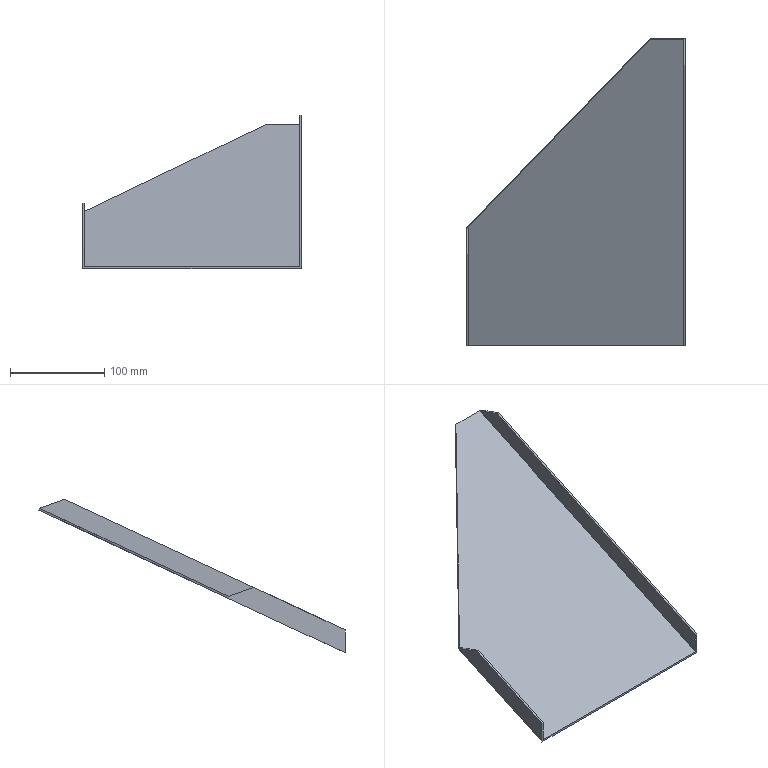Part | NX | features solid 2 | 1 solid | 13 faces | box 232.306 x 325 x 163.036 mm | volume 141866 mm3 | plane 13
STEP:
#1=CARTESIAN_POINT('',(339.694,-556.33,-245.421));
#2=VERTEX_POINT('',#1);
#3=CARTESIAN_POINT('',(337.694,-556.33,-245.421));
#4=VERTEX_POINT('',#3);
#5=CARTESIAN_POINT('',(337.694,-556.33,-245.421));
#6=DIRECTION('',(1.,0.,0.));
#7=VECTOR('',#6,1000.);
#8=LINE('',#5,#7);
#9=EDGE_CURVE('',#2,#4,#8,.F.);
#10=ORIENTED_EDGE('',*,*,#9,.F.);
#11=CARTESIAN_POINT('',(339.694,-680.,-303.09));
#12=VERTEX_POINT('',#11);
#13=CARTESIAN_POINT('',(339.694,-556.33,-245.421));
#14=DIRECTION('',(0.,-0.9063,-0.4226));
#15=VECTOR('',#14,1000.);
#16=LINE('',#13,#15);
#17=EDGE_CURVE('',#2,#12,#16,.T.);
#18=ORIENTED_EDGE('',*,*,#17,.T.);
#19=CARTESIAN_POINT('',(568.,-680.,-303.09));
#20=VERTEX_POINT('',#19);
#21=CARTESIAN_POINT('',(188.564,-680.,-303.09));
#22=DIRECTION('',(1.,0.,0.));
#23=VECTOR('',#22,1000.);
#24=LINE('',#21,#23);
#25=EDGE_CURVE('',#20,#12,#24,.F.);
#26=ORIENTED_EDGE('',*,*,#25,.F.);
#27=CARTESIAN_POINT('',(568.,-355.845,-151.934));
#28=VERTEX_POINT('',#27);
#29=CARTESIAN_POINT('',(568.,-355.845,-151.934));
#30=DIRECTION('',(0.,-0.9063,-0.4226));
#31=VECTOR('',#30,1000.);
#32=LINE('',#29,#31);
#33=EDGE_CURVE('',#28,#20,#32,.T.);
#34=ORIENTED_EDGE('',*,*,#33,.F.);
#35=CARTESIAN_POINT('',(532.61,-355.845,-151.934));
#36=VERTEX_POINT('',#35);
#37=CARTESIAN_POINT('',(570.,-355.845,-151.934));
#38=DIRECTION('',(-1.,0.,0.));
#39=VECTOR('',#38,1000.);
#40=LINE('',#37,#39);
#41=EDGE_CURVE('',#28,#36,#40,.T.);
#42=ORIENTED_EDGE('',*,*,#41,.T.);
#43=CARTESIAN_POINT('',(554.599,-333.228,-141.387));
#44=DIRECTION('',(-0.6611,-0.68,-0.3171));
#45=VECTOR('',#44,1000.);
#46=LINE('',#43,#45);
#47=EDGE_CURVE('',#36,#4,#46,.T.);
#48=ORIENTED_EDGE('',*,*,#47,.T.);
#49=EDGE_LOOP('',(#10,#18,#26,#34,#42,#48));
#50=FACE_BOUND('',#49,.T.);
#51=CARTESIAN_POINT('',(337.694,-522.729,-229.753));
#52=DIRECTION('',(0.,-0.4226,0.9063));
#53=DIRECTION('',(1.,0.,0.));
#54=AXIS2_PLACEMENT_3D('',#51,#52,#53);
#55=PLANE('',#54);
#56=ADVANCED_FACE('',(#50),#55,.T.);
#57=CARTESIAN_POINT('',(570.,-355.,-153.747));
#58=VERTEX_POINT('',#57);
#59=CARTESIAN_POINT('',(532.61,-355.,-153.747));
#60=VERTEX_POINT('',#59);
#61=CARTESIAN_POINT('',(570.,-355.,-153.747));
#62=DIRECTION('',(-1.,0.,0.));
#63=VECTOR('',#62,1000.);
#64=LINE('',#61,#63);
#65=EDGE_CURVE('',#58,#60,#64,.T.);
#66=ORIENTED_EDGE('',*,*,#65,.T.);
#67=CARTESIAN_POINT('',(532.61,-355.845,-151.934));
#68=DIRECTION('',(0.,0.4226,-0.9063));
#69=VECTOR('',#68,1000.);
#70=LINE('',#67,#69);
#71=EDGE_CURVE('',#36,#60,#70,.T.);
#72=ORIENTED_EDGE('',*,*,#71,.F.);
#73=ORIENTED_EDGE('',*,*,#41,.F.);
#74=CARTESIAN_POINT('',(570.,-355.845,-151.934));
#75=VERTEX_POINT('',#74);
#76=CARTESIAN_POINT('',(570.,-355.845,-151.934));
#77=DIRECTION('',(-1.,0.,0.));
#78=VECTOR('',#77,1000.);
#79=LINE('',#76,#78);
#80=EDGE_CURVE('',#75,#28,#79,.T.);
#81=ORIENTED_EDGE('',*,*,#80,.F.);
#82=CARTESIAN_POINT('',(570.,-355.845,-151.934));
#83=DIRECTION('',(0.,0.4226,-0.9063));
#84=VECTOR('',#83,1000.);
#85=LINE('',#82,#84);
#86=EDGE_CURVE('',#75,#58,#85,.T.);
#87=ORIENTED_EDGE('',*,*,#86,.T.);
#88=EDGE_LOOP('',(#66,#72,#73,#81,#87));
#89=FACE_BOUND('',#88,.T.);
#90=CARTESIAN_POINT('',(570.,-355.845,-151.934));
#91=DIRECTION('',(0.,-0.9063,-0.4226));
#92=DIRECTION('',(0.,0.4226,-0.9063));
#93=AXIS2_PLACEMENT_3D('',#90,#91,#92);
#94=PLANE('',#93);
#95=ADVANCED_FACE('',(#89),#94,.F.);
#96=CARTESIAN_POINT('',(337.694,-555.485,-247.234));
#97=VERTEX_POINT('',#96);
#98=CARTESIAN_POINT('',(554.599,-332.383,-143.2));
#99=DIRECTION('',(-0.6611,-0.68,-0.3171));
#100=VECTOR('',#99,1000.);
#101=LINE('',#98,#100);
#102=EDGE_CURVE('',#60,#97,#101,.T.);
#103=ORIENTED_EDGE('',*,*,#102,.T.);
#104=CARTESIAN_POINT('',(337.694,-556.33,-245.421));
#105=DIRECTION('',(0.,0.4226,-0.9063));
#106=VECTOR('',#105,1000.);
#107=LINE('',#104,#106);
#108=EDGE_CURVE('',#4,#97,#107,.T.);
#109=ORIENTED_EDGE('',*,*,#108,.F.);
#110=ORIENTED_EDGE('',*,*,#47,.F.);
#111=ORIENTED_EDGE('',*,*,#71,.T.);
#112=EDGE_LOOP('',(#103,#109,#110,#111));
#113=FACE_BOUND('',#112,.T.);
#114=CARTESIAN_POINT('',(554.599,-333.228,-141.387));
#115=DIRECTION('',(0.7503,-0.5992,-0.2794));
#116=DIRECTION('',(0.624,0.7814,0.));
#117=AXIS2_PLACEMENT_3D('',#114,#115,#116);
#118=PLANE('',#117);
#119=ADVANCED_FACE('',(#113),#118,.F.);
#120=CARTESIAN_POINT('',(337.694,-680.,-305.297));
#121=VERTEX_POINT('',#120);
#122=CARTESIAN_POINT('',(337.694,-479.94,-212.007));
#123=DIRECTION('',(0.,-0.9063,-0.4226));
#124=VECTOR('',#123,1000.);
#125=LINE('',#122,#124);
#126=EDGE_CURVE('',#97,#121,#125,.T.);
#127=ORIENTED_EDGE('',*,*,#126,.T.);
#128=CARTESIAN_POINT('',(337.694,-680.,-281.022));
#129=VERTEX_POINT('',#128);
#130=CARTESIAN_POINT('',(337.694,-680.,-210.194));
#131=DIRECTION('',(0.,0.,1.));
#132=VECTOR('',#131,1000.);
#133=LINE('',#130,#132);
#134=EDGE_CURVE('',#129,#121,#133,.F.);
#135=ORIENTED_EDGE('',*,*,#134,.F.);
#136=CARTESIAN_POINT('',(337.694,-582.908,-235.748));
#137=VERTEX_POINT('',#136);
#138=CARTESIAN_POINT('',(337.694,-564.782,-227.295));
#139=DIRECTION('',(0.,-0.9063,-0.4226));
#140=VECTOR('',#139,1000.);
#141=LINE('',#138,#140);
#142=EDGE_CURVE('',#137,#129,#141,.T.);
#143=ORIENTED_EDGE('',*,*,#142,.F.);
#144=CARTESIAN_POINT('',(337.694,-556.33,-245.421));
#145=DIRECTION('',(0.,-0.9397,0.342));
#146=VECTOR('',#145,1000.);
#147=LINE('',#144,#146);
#148=EDGE_CURVE('',#137,#4,#147,.F.);
#149=ORIENTED_EDGE('',*,*,#148,.T.);
#150=ORIENTED_EDGE('',*,*,#108,.T.);
#151=EDGE_LOOP('',(#127,#135,#143,#149,#150));
#152=FACE_BOUND('',#151,.T.);
#153=CARTESIAN_POINT('',(337.694,-480.785,-210.194));
#154=DIRECTION('',(1.,0.,0.));
#155=DIRECTION('',(0.,1.,0.));
#156=AXIS2_PLACEMENT_3D('',#153,#154,#155);
#157=PLANE('',#156);
#158=ADVANCED_FACE('',(#152),#157,.F.);
#159=CARTESIAN_POINT('',(570.,-680.,-305.297));
#160=VERTEX_POINT('',#159);
#161=CARTESIAN_POINT('',(188.564,-680.,-305.297));
#162=DIRECTION('',(1.,0.,0.));
#163=VECTOR('',#162,1000.);
#164=LINE('',#161,#163);
#165=EDGE_CURVE('',#160,#121,#164,.F.);
#166=ORIENTED_EDGE('',*,*,#165,.F.);
#167=CARTESIAN_POINT('',(570.,-680.,-281.022));
#168=VERTEX_POINT('',#167);
#169=CARTESIAN_POINT('',(570.,-680.,234.426));
#170=DIRECTION('',(0.,0.,1.));
#171=VECTOR('',#170,1000.);
#172=LINE('',#169,#171);
#173=EDGE_CURVE('',#168,#160,#172,.F.);
#174=ORIENTED_EDGE('',*,*,#173,.F.);
#175=CARTESIAN_POINT('',(568.,-680.,-281.022));
#176=VERTEX_POINT('',#175);
#177=CARTESIAN_POINT('',(570.,-680.,-281.022));
#178=DIRECTION('',(1.,0.,0.));
#179=VECTOR('',#178,1000.);
#180=LINE('',#177,#179);
#181=EDGE_CURVE('',#176,#168,#180,.T.);
#182=ORIENTED_EDGE('',*,*,#181,.F.);
#183=CARTESIAN_POINT('',(568.,-680.,-151.934));
#184=DIRECTION('',(0.,0.,-1.));
#185=VECTOR('',#184,1000.);
#186=LINE('',#183,#185);
#187=EDGE_CURVE('',#20,#176,#186,.F.);
#188=ORIENTED_EDGE('',*,*,#187,.F.);
#189=ORIENTED_EDGE('',*,*,#25,.T.);
#190=CARTESIAN_POINT('',(339.694,-680.,-281.022));
#191=VERTEX_POINT('',#190);
#192=CARTESIAN_POINT('',(339.694,-680.,-430.));
#193=DIRECTION('',(0.,0.,1.));
#194=VECTOR('',#193,1000.);
#195=LINE('',#192,#194);
#196=EDGE_CURVE('',#12,#191,#195,.T.);
#197=ORIENTED_EDGE('',*,*,#196,.T.);
#198=CARTESIAN_POINT('',(188.564,-680.,-281.022));
#199=DIRECTION('',(-1.,0.,0.));
#200=VECTOR('',#199,1000.);
#201=LINE('',#198,#200);
#202=EDGE_CURVE('',#191,#129,#201,.T.);
#203=ORIENTED_EDGE('',*,*,#202,.T.);
#204=ORIENTED_EDGE('',*,*,#134,.T.);
#205=EDGE_LOOP('',(#166,#174,#182,#188,#189,#197,#203,#204));
#206=FACE_BOUND('',#205,.T.);
#207=CARTESIAN_POINT('',(188.564,-680.,-430.));
#208=DIRECTION('',(0.,1.,0.));
#209=DIRECTION('',(-1.,0.,0.));
#210=AXIS2_PLACEMENT_3D('',#207,#208,#209);
#211=PLANE('',#210);
#212=ADVANCED_FACE('',(#206),#211,.F.);
#213=CARTESIAN_POINT('',(570.,473.552,232.614));
#214=DIRECTION('',(0.,-0.9063,-0.4226));
#215=VECTOR('',#214,1000.);
#216=LINE('',#213,#215);
#217=EDGE_CURVE('',#58,#160,#216,.T.);
#218=ORIENTED_EDGE('',*,*,#217,.F.);
#219=ORIENTED_EDGE('',*,*,#86,.F.);
#220=CARTESIAN_POINT('',(570.,-382.424,-142.26));
#221=VERTEX_POINT('',#220);
#222=CARTESIAN_POINT('',(570.,-355.845,-151.934));
#223=DIRECTION('',(0.,0.9397,-0.342));
#224=VECTOR('',#223,1000.);
#225=LINE('',#222,#224);
#226=EDGE_CURVE('',#75,#221,#225,.F.);
#227=ORIENTED_EDGE('',*,*,#226,.T.);
#228=CARTESIAN_POINT('',(570.,-364.298,-133.808));
#229=DIRECTION('',(0.,-0.9063,-0.4226));
#230=VECTOR('',#229,1000.);
#231=LINE('',#228,#230);
#232=EDGE_CURVE('',#221,#168,#231,.T.);
#233=ORIENTED_EDGE('',*,*,#232,.T.);
#234=ORIENTED_EDGE('',*,*,#173,.T.);
#235=EDGE_LOOP('',(#218,#219,#227,#233,#234));
#236=FACE_BOUND('',#235,.T.);
#237=CARTESIAN_POINT('',(570.,472.707,234.426));
#238=DIRECTION('',(1.,0.,0.));
#239=DIRECTION('',(0.,0.,-1.));
#240=AXIS2_PLACEMENT_3D('',#237,#238,#239);
#241=PLANE('',#240);
#242=ADVANCED_FACE('',(#236),#241,.T.);
#243=ORIENTED_EDGE('',*,*,#65,.F.);
#244=ORIENTED_EDGE('',*,*,#217,.T.);
#245=ORIENTED_EDGE('',*,*,#165,.T.);
#246=ORIENTED_EDGE('',*,*,#126,.F.);
#247=ORIENTED_EDGE('',*,*,#102,.F.);
#248=EDGE_LOOP('',(#243,#244,#245,#246,#247));
#249=FACE_BOUND('',#248,.T.);
#250=CARTESIAN_POINT('',(337.694,-521.883,-231.565));
#251=DIRECTION('',(0.,-0.4226,0.9063));
#252=DIRECTION('',(1.,0.,0.));
#253=AXIS2_PLACEMENT_3D('',#250,#251,#252);
#254=PLANE('',#253);
#255=ADVANCED_FACE('',(#249),#254,.F.);
#256=ORIENTED_EDGE('',*,*,#232,.F.);
#257=CARTESIAN_POINT('',(568.,-382.424,-142.26));
#258=VERTEX_POINT('',#257);
#259=CARTESIAN_POINT('',(570.,-382.424,-142.26));
#260=DIRECTION('',(1.,0.,0.));
#261=VECTOR('',#260,1000.);
#262=LINE('',#259,#261);
#263=EDGE_CURVE('',#221,#258,#262,.F.);
#264=ORIENTED_EDGE('',*,*,#263,.T.);
#265=CARTESIAN_POINT('',(568.,-364.298,-133.808));
#266=DIRECTION('',(0.,-0.9063,-0.4226));
#267=VECTOR('',#266,1000.);
#268=LINE('',#265,#267);
#269=EDGE_CURVE('',#258,#176,#268,.T.);
#270=ORIENTED_EDGE('',*,*,#269,.T.);
#271=ORIENTED_EDGE('',*,*,#181,.T.);
#272=EDGE_LOOP('',(#256,#264,#270,#271));
#273=FACE_BOUND('',#272,.T.);
#274=CARTESIAN_POINT('',(570.,-364.298,-133.808));
#275=DIRECTION('',(0.,0.4226,-0.9063));
#276=DIRECTION('',(0.,-0.9063,-0.4226));
#277=AXIS2_PLACEMENT_3D('',#274,#275,#276);
#278=PLANE('',#277);
#279=ADVANCED_FACE('',(#273),#278,.F.);
#280=ORIENTED_EDGE('',*,*,#269,.F.);
#281=CARTESIAN_POINT('',(568.,-355.845,-151.934));
#282=DIRECTION('',(0.,-0.9397,0.342));
#283=VECTOR('',#282,1000.);
#284=LINE('',#281,#283);
#285=EDGE_CURVE('',#258,#28,#284,.F.);
#286=ORIENTED_EDGE('',*,*,#285,.T.);
#287=ORIENTED_EDGE('',*,*,#33,.T.);
#288=ORIENTED_EDGE('',*,*,#187,.T.);
#289=EDGE_LOOP('',(#280,#286,#287,#288));
#290=FACE_BOUND('',#289,.T.);
#291=CARTESIAN_POINT('',(568.,-355.845,-151.934));
#292=DIRECTION('',(-1.,0.,0.));
#293=DIRECTION('',(0.,0.,1.));
#294=AXIS2_PLACEMENT_3D('',#291,#292,#293);
#295=PLANE('',#294);
#296=ADVANCED_FACE('',(#290),#295,.T.);
#297=ORIENTED_EDGE('',*,*,#285,.F.);
#298=ORIENTED_EDGE('',*,*,#263,.F.);
#299=ORIENTED_EDGE('',*,*,#226,.F.);
#300=ORIENTED_EDGE('',*,*,#80,.T.);
#301=EDGE_LOOP('',(#297,#298,#299,#300));
#302=FACE_BOUND('',#301,.T.);
#303=CARTESIAN_POINT('',(570.,-355.845,-151.934));
#304=DIRECTION('',(0.,-0.342,-0.9397));
#305=DIRECTION('',(0.,0.9397,-0.342));
#306=AXIS2_PLACEMENT_3D('',#303,#304,#305);
#307=PLANE('',#306);
#308=ADVANCED_FACE('',(#302),#307,.F.);
#309=CARTESIAN_POINT('',(339.694,-582.908,-235.748));
#310=VERTEX_POINT('',#309);
#311=CARTESIAN_POINT('',(339.694,-564.782,-227.295));
#312=DIRECTION('',(0.,-0.9063,-0.4226));
#313=VECTOR('',#312,1000.);
#314=LINE('',#311,#313);
#315=EDGE_CURVE('',#310,#191,#314,.T.);
#316=ORIENTED_EDGE('',*,*,#315,.F.);
#317=CARTESIAN_POINT('',(337.694,-582.908,-235.748));
#318=DIRECTION('',(-1.,0.,0.));
#319=VECTOR('',#318,1000.);
#320=LINE('',#317,#319);
#321=EDGE_CURVE('',#310,#137,#320,.T.);
#322=ORIENTED_EDGE('',*,*,#321,.T.);
#323=ORIENTED_EDGE('',*,*,#142,.T.);
#324=ORIENTED_EDGE('',*,*,#202,.F.);
#325=EDGE_LOOP('',(#316,#322,#323,#324));
#326=FACE_BOUND('',#325,.T.);
#327=CARTESIAN_POINT('',(337.694,-564.782,-227.295));
#328=DIRECTION('',(0.,0.4226,-0.9063));
#329=DIRECTION('',(0.,-0.9063,-0.4226));
#330=AXIS2_PLACEMENT_3D('',#327,#328,#329);
#331=PLANE('',#330);
#332=ADVANCED_FACE('',(#326),#331,.F.);
#333=ORIENTED_EDGE('',*,*,#17,.F.);
#334=CARTESIAN_POINT('',(339.694,-582.908,-235.748));
#335=DIRECTION('',(0.,0.9397,-0.342));
#336=VECTOR('',#335,1000.);
#337=LINE('',#334,#336);
#338=EDGE_CURVE('',#2,#310,#337,.F.);
#339=ORIENTED_EDGE('',*,*,#338,.T.);
#340=ORIENTED_EDGE('',*,*,#315,.T.);
#341=ORIENTED_EDGE('',*,*,#196,.F.);
#342=EDGE_LOOP('',(#333,#339,#340,#341));
#343=FACE_BOUND('',#342,.T.);
#344=CARTESIAN_POINT('',(339.694,-556.33,-245.421));
#345=DIRECTION('',(-1.,0.,0.));
#346=DIRECTION('',(0.,-1.,0.));
#347=AXIS2_PLACEMENT_3D('',#344,#345,#346);
#348=PLANE('',#347);
#349=ADVANCED_FACE('',(#343),#348,.F.);
#350=ORIENTED_EDGE('',*,*,#338,.F.);
#351=ORIENTED_EDGE('',*,*,#9,.T.);
#352=ORIENTED_EDGE('',*,*,#148,.F.);
#353=ORIENTED_EDGE('',*,*,#321,.F.);
#354=EDGE_LOOP('',(#350,#351,#352,#353));
#355=FACE_BOUND('',#354,.T.);
#356=CARTESIAN_POINT('',(337.694,-582.908,-235.748));
#357=DIRECTION('',(0.,-0.342,-0.9397));
#358=DIRECTION('',(0.,0.9397,-0.342));
#359=AXIS2_PLACEMENT_3D('',#356,#357,#358);
#360=PLANE('',#359);
#361=ADVANCED_FACE('',(#355),#360,.F.);
#362=CLOSED_SHELL('',(#56,#95,#119,#158,#212,#242,#255,#279,#296,#308,#332,#349,#361));
#363=MANIFOLD_SOLID_BREP('',#362);
#364=(LENGTH_UNIT()NAMED_UNIT(*)SI_UNIT(.MILLI.,.METRE.));
#365=UNCERTAINTY_MEASURE_WITH_UNIT(LENGTH_MEASURE(0.00001),#364,'','');
#366=(NAMED_UNIT(*)PLANE_ANGLE_UNIT()SI_UNIT($,.RADIAN.));
#367=(NAMED_UNIT(*)SI_UNIT($,.STERADIAN.)SOLID_ANGLE_UNIT());
#368=(GEOMETRIC_REPRESENTATION_CONTEXT(3)GLOBAL_UNCERTAINTY_ASSIGNED_CONTEXT((#365))GLOBAL_UNIT_ASSIGNED_CONTEXT((#364,#366,#367))REPRESENTATION_CONTEXT('',''));
#369=ADVANCED_BREP_SHAPE_REPRESENTATION('',(#363),#368);